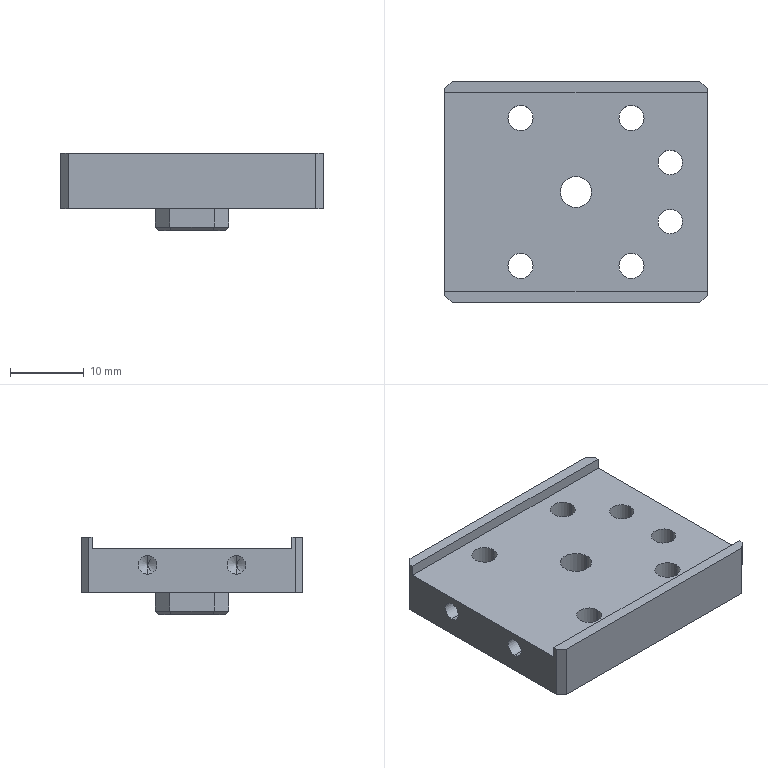Part | SolidWorks | features HoleWzd 4, Chamfer 3, Cut 1, Extrusion 1, ICE 1 | 1 solid | 67 faces | box 35.5 x 30 x 10.5 mm | volume 5956 mm3 | plane 35 | cylinder 26 | cone 6 | commonest cylinder face diameters 3.4 x8 6.5 x8 2.5 x4 3.3 x4 4.2 x2